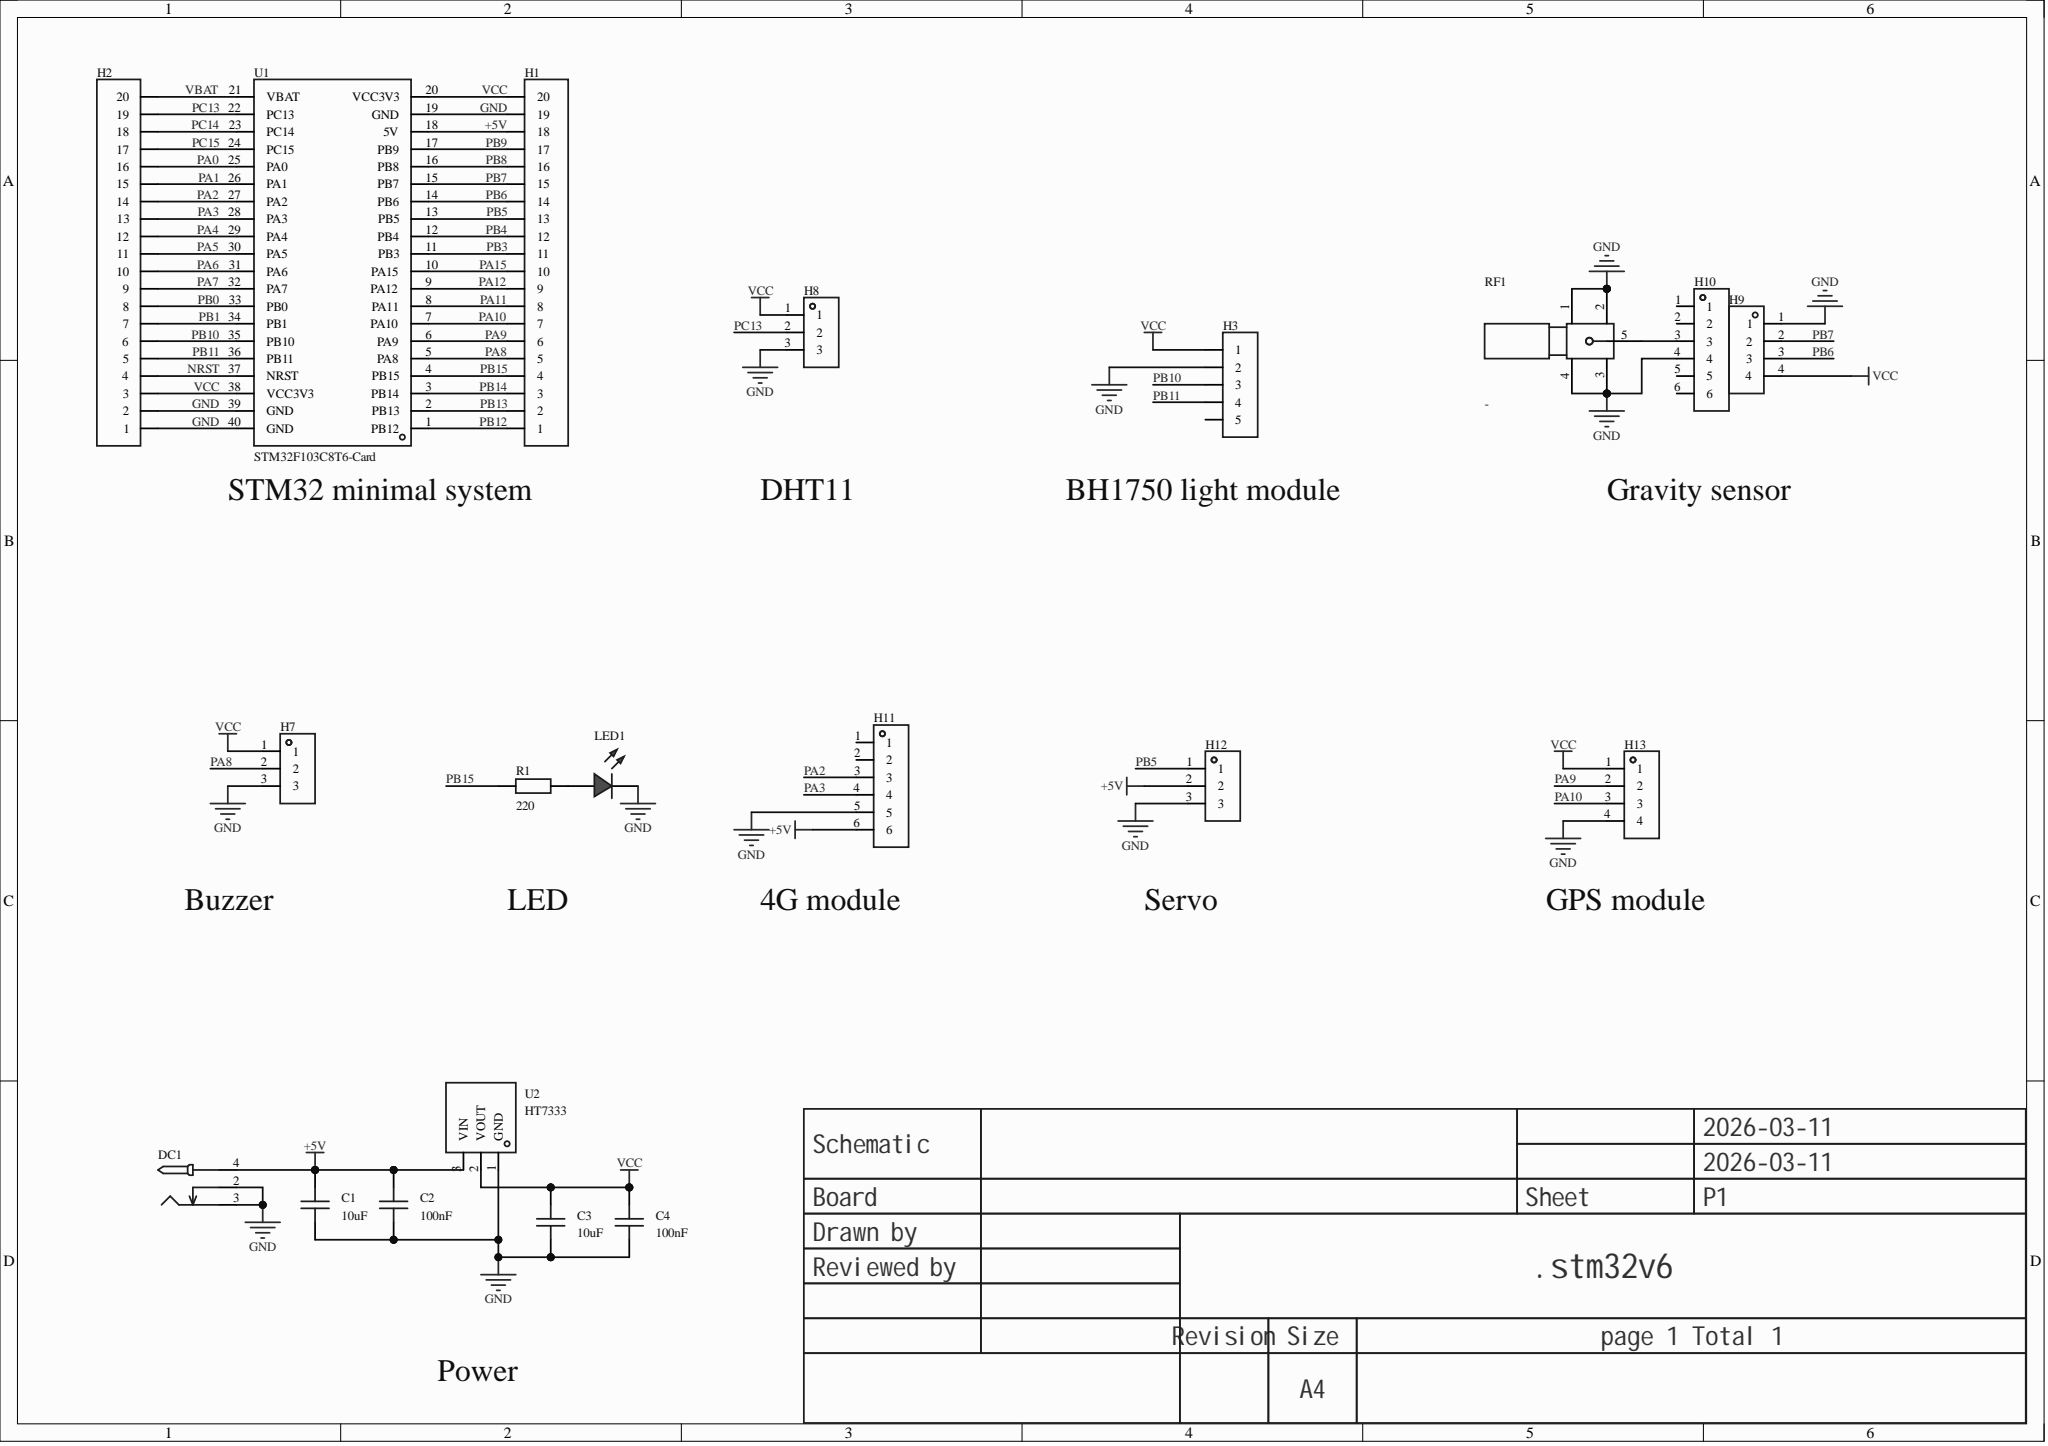Circuit board | Altium Designer | 20 parts | 39 nets
Bill of materials:
Comment,Description,Designator,Footprint,LibRef,Quantity
"10uF","","C1, C3","C0603","CAP_0603","2"
"100nF","","C2, C4","C0603","CAP_0603","2"
"","","DC1","DC-2.0","DC-005_2.0","1"
"","","H1, H2","HDR-TH_20P-P2.54-V-F","HDR-F_2.54_1x20P","2"
"","","H3","HDR-TH_5P-P2.54-V-F","HDR-F_2.54_1x5P","1"
"","","H7, H8","HDR-TH_3P-P2.54-V-F","HDR-F_2.54_1x3P","2"
"","","H9, H13","HDR-TH_4P-P2.54-V-F","HDR-F_2.54_1x4P","2"
"","","H10, H11","HDR-TH_6P-P2.54-V-F","HDR-F_2.54_1x6P","2"
"","","H12","HDR-TH_3P-P2.54-V-M","HDR-M_2.54_1x3P","1"
"","","LED1","LED_TH-3mm","LED_TH-R_3mm","1"
"220","","R1","Res_1/8W","Res_AXIAL-1/8W","1"
"-","Connector type: board mount; Interface type: inner hole; Number of ports: 1; Interface diameter: 5.2mm; Interface length/height: -; Frequency: -; RF series: SMA; Impedance: 50O; Style: right angle; Operating temperature: -;","RF1","SMA-SMD_BWSMA-KE-P001","BWSMA-KE-P001","1"
"STM32F103C8T6-Card","","U1","CONN-TH_L53.3-W22.9_STM32F103C8T6-CARD","STM32F103C8T6-Card","1"
"HT7333","Output type: fixed; Operating voltage: 12V; Output voltage: 3.3V; Output current: 250mA; PSRR: -; Output polarity: positive;","U2","SOT-23-3_L2.9-W1.6-P1.90-LS2.8-BR","HT7333","1"
Netlist (Protel format):
[
C1
C0603
10uF



]
[
C2
C0603
100nF



]
[
C3
C0603
10uF



]
[
C4
C0603
100nF



]
[
DC1
DC-2.0




]
[
H1
HDR-TH_20P-P2.54-V-F




]
[
H2
HDR-TH_20P-P2.54-V-F




]
[
H3
HDR-TH_5P-P2.54-V-F




]
[
H7
HDR-TH_3P-P2.54-V-F




]
[
H8
HDR-TH_3P-P2.54-V-F




]
[
H9
HDR-TH_4P-P2.54-V-F




]
[
H10
HDR-TH_6P-P2.54-V-F




]
[
H11
HDR-TH_6P-P2.54-V-F




]
[
H12
HDR-TH_3P-P2.54-V-M




]
[
H13
HDR-TH_4P-P2.54-V-F




]
[
LED1
LED_TH-3mm




]
[
R1
Res_1/8W
220



]
[
RF1
SMA-SMD_BWSMA-KE-P001
-



]
[
U1
CONN-TH_L53.3-W22.9_STM32F103C8T6-CARD
STM32F103C8T6-Card



]
[
U2
SOT-23-3_L2.9-W1.6-P1.90-LS2.8-BR
HT7333



]
(
VCC
C3-2
C4-2
H1-20
H2-3
H3-1
H7-1
H8-1
H9-4
H13-1
U1-20
U1-38
U2-2
)
(
VBAT
H2-20
U1-21
)
(
PC15
H2-17
U1-24
)
(
PC14
H2-18
U1-23
)
(
PC13
H2-19
H8-2
U1-22
)
(
PB15
H1-4
R1-1
U1-4
)
(
PB14
H1-3
U1-3
)
(
PB13
H1-2
U1-2
)
(
PB12
H1-1
U1-1
)
(
PB11
H2-5
H3-4
U1-36
)
(
PB10
H2-6
H3-3
U1-35
)
(
PB9
H1-17
U1-17
)
(
PB8
H1-16
U1-16
)
(
PB7
H1-15
H9-2
U1-15
)
(
PB6
H1-14
H9-3
U1-14
)
(
PB5
H1-13
H12-1
U1-13
)
(
PB4
H1-12
U1-12
)
(
PB3
H1-11
U1-11
)
(
PB1
H2-7
U1-34
)
(
PB0
H2-8
U1-33
)
(
PA15
H1-10
U1-10
)
(
PA12
H1-9
U1-9
)
(
PA11
H1-8
U1-8
)
(
PA10
H1-7
H13-3
U1-7
)
(
PA9
H1-6
H13-2
U1-6
)
(
PA8
H1-5
H7-2
U1-5
)
(
PA7
H2-9
U1-32
)
(
PA6
H2-10
U1-31
)
(
PA5
H2-11
U1-30
)
(
PA4
H2-12
U1-29
)
(
PA3
H2-13
H11-4
U1-28
)
(
PA2
H2-14
H11-3
U1-27
)
(
PA1
H2-15
U1-26
)
(
PA0
H2-16
U1-25
)
(
NRST
H2-4
U1-37
)
(
NetLED1_1
LED1-1
R1-2
)
(
NetH10_3
H10-3
RF1-5
)
(
GND
C1-1
C2-1
C3-1
C4-1
DC1-2
DC1-3
H1-19
H2-1
H2-2
H3-2
H7-3
H8-3
H9-1
H10-4
H11-5
H12-3
H13-4
LED1-2
RF1-1
RF1-2
RF1-3
RF1-4
U1-19
U1-39
U1-40
U2-1
)
(
+5V
C1-2
C2-2
DC1-4
H1-18
H11-6
H12-2
U1-18
U2-3
)